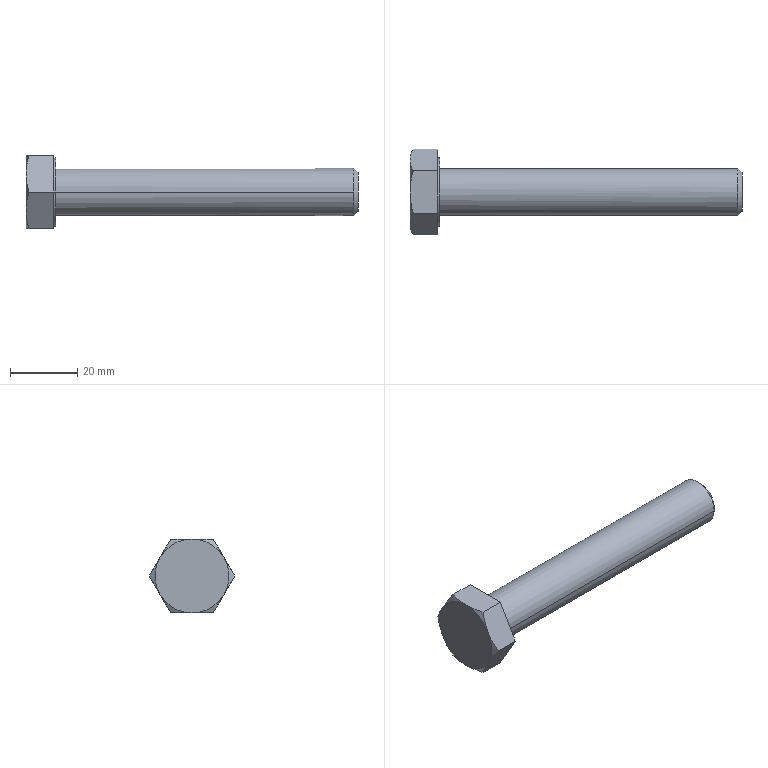Part | STEP file | DIN 931-1 - M14 x 90 | 1 solid | 22 faces | box 98.8 x 25.403 x 22 mm | volume 17447 mm3 | plane 10 | cone 8 | cylinder 4 | commonest cylinder face diameters 14 x2 20.5 x2